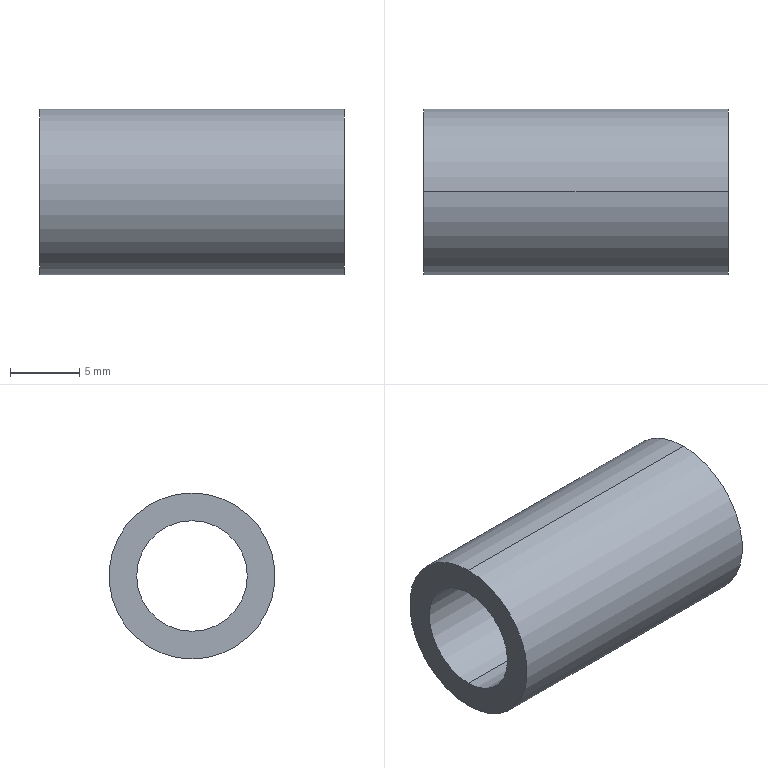Part | SolidWorks | features Revolution 1 | 1 solid | 6 faces | box 22 x 12 x 12 mm | volume 1382 mm3 | cylinder 4 | plane 2 | commonest cylinder face diameters 8 x2 12 x2
STEP:
#1=CARTESIAN_POINT('',(22.,0.,6.));
#2=VERTEX_POINT('',#1);
#3=CARTESIAN_POINT('',(22.,0.,-6.));
#4=VERTEX_POINT('',#3);
#5=CARTESIAN_POINT('',(22.,0.,0.));
#6=DIRECTION('',(-1.,0.,0.));
#7=DIRECTION('',(0.,0.,1.));
#8=AXIS2_PLACEMENT_3D('',#5,#6,#7);
#9=CIRCLE('',#8,6.);
#10=EDGE_CURVE('',#2,#4,#9,.T.);
#11=ORIENTED_EDGE('',*,*,#10,.T.);
#12=CARTESIAN_POINT('',(0.,0.,-6.));
#13=VERTEX_POINT('',#12);
#14=CARTESIAN_POINT('',(-539.036,0.,-6.));
#15=DIRECTION('',(-1.,0.,0.));
#16=VECTOR('',#15,1000.);
#17=LINE('',#14,#16);
#18=EDGE_CURVE('',#4,#13,#17,.T.);
#19=ORIENTED_EDGE('',*,*,#18,.T.);
#20=CARTESIAN_POINT('',(0.,0.,6.));
#21=VERTEX_POINT('',#20);
#22=CARTESIAN_POINT('',(0.,0.,0.));
#23=DIRECTION('',(-1.,0.,0.));
#24=DIRECTION('',(0.,0.,1.));
#25=AXIS2_PLACEMENT_3D('',#22,#23,#24);
#26=CIRCLE('',#25,6.);
#27=EDGE_CURVE('',#21,#13,#26,.T.);
#28=ORIENTED_EDGE('',*,*,#27,.F.);
#29=CARTESIAN_POINT('',(-539.036,0.,6.));
#30=DIRECTION('',(-1.,0.,0.));
#31=VECTOR('',#30,1000.);
#32=LINE('',#29,#31);
#33=EDGE_CURVE('',#2,#21,#32,.T.);
#34=ORIENTED_EDGE('',*,*,#33,.F.);
#35=EDGE_LOOP('',(#11,#19,#28,#34));
#36=FACE_OUTER_BOUND('',#35,.T.);
#37=CARTESIAN_POINT('',(-539.036,0.,0.));
#38=DIRECTION('',(-1.,0.,0.));
#39=DIRECTION('',(0.,0.,1.));
#40=AXIS2_PLACEMENT_3D('',#37,#38,#39);
#41=CYLINDRICAL_SURFACE('',#40,6.);
#42=ADVANCED_FACE('',(#36),#41,.T.);
#43=CARTESIAN_POINT('',(22.,0.,-4.));
#44=VERTEX_POINT('',#43);
#45=CARTESIAN_POINT('',(22.,0.,4.));
#46=VERTEX_POINT('',#45);
#47=CARTESIAN_POINT('',(22.,0.,0.));
#48=DIRECTION('',(-1.,0.,0.));
#49=DIRECTION('',(0.,0.,1.));
#50=AXIS2_PLACEMENT_3D('',#47,#48,#49);
#51=CIRCLE('',#50,4.);
#52=EDGE_CURVE('',#44,#46,#51,.T.);
#53=ORIENTED_EDGE('',*,*,#52,.F.);
#54=CARTESIAN_POINT('',(0.,0.,-4.));
#55=VERTEX_POINT('',#54);
#56=CARTESIAN_POINT('',(-539.036,0.,-4.));
#57=DIRECTION('',(-1.,0.,0.));
#58=VECTOR('',#57,1000.);
#59=LINE('',#56,#58);
#60=EDGE_CURVE('',#44,#55,#59,.T.);
#61=ORIENTED_EDGE('',*,*,#60,.T.);
#62=CARTESIAN_POINT('',(0.,0.,4.));
#63=VERTEX_POINT('',#62);
#64=CARTESIAN_POINT('',(0.,0.,0.));
#65=DIRECTION('',(-1.,0.,0.));
#66=DIRECTION('',(0.,0.,1.));
#67=AXIS2_PLACEMENT_3D('',#64,#65,#66);
#68=CIRCLE('',#67,4.);
#69=EDGE_CURVE('',#55,#63,#68,.T.);
#70=ORIENTED_EDGE('',*,*,#69,.T.);
#71=CARTESIAN_POINT('',(-539.036,0.,4.));
#72=DIRECTION('',(-1.,0.,0.));
#73=VECTOR('',#72,1000.);
#74=LINE('',#71,#73);
#75=EDGE_CURVE('',#46,#63,#74,.T.);
#76=ORIENTED_EDGE('',*,*,#75,.F.);
#77=EDGE_LOOP('',(#53,#61,#70,#76));
#78=FACE_OUTER_BOUND('',#77,.T.);
#79=CARTESIAN_POINT('',(-539.036,0.,0.));
#80=DIRECTION('',(-1.,0.,0.));
#81=DIRECTION('',(0.,0.,1.));
#82=AXIS2_PLACEMENT_3D('',#79,#80,#81);
#83=CYLINDRICAL_SURFACE('',#82,4.);
#84=ADVANCED_FACE('',(#78),#83,.F.);
#85=ORIENTED_EDGE('',*,*,#60,.F.);
#86=CARTESIAN_POINT('',(22.,0.,0.));
#87=DIRECTION('',(-1.,0.,0.));
#88=DIRECTION('',(0.,0.,1.));
#89=AXIS2_PLACEMENT_3D('',#86,#87,#88);
#90=CIRCLE('',#89,4.);
#91=EDGE_CURVE('',#46,#44,#90,.T.);
#92=ORIENTED_EDGE('',*,*,#91,.F.);
#93=ORIENTED_EDGE('',*,*,#75,.T.);
#94=CARTESIAN_POINT('',(0.,0.,0.));
#95=DIRECTION('',(-1.,0.,0.));
#96=DIRECTION('',(0.,0.,1.));
#97=AXIS2_PLACEMENT_3D('',#94,#95,#96);
#98=CIRCLE('',#97,4.);
#99=EDGE_CURVE('',#63,#55,#98,.T.);
#100=ORIENTED_EDGE('',*,*,#99,.T.);
#101=EDGE_LOOP('',(#85,#92,#93,#100));
#102=FACE_OUTER_BOUND('',#101,.T.);
#103=CARTESIAN_POINT('',(-539.036,0.,0.));
#104=DIRECTION('',(-1.,0.,0.));
#105=DIRECTION('',(0.,0.,1.));
#106=AXIS2_PLACEMENT_3D('',#103,#104,#105);
#107=CYLINDRICAL_SURFACE('',#106,4.);
#108=ADVANCED_FACE('',(#102),#107,.F.);
#109=ORIENTED_EDGE('',*,*,#99,.F.);
#110=ORIENTED_EDGE('',*,*,#69,.F.);
#111=EDGE_LOOP('',(#109,#110));
#112=FACE_BOUND('',#111,.T.);
#113=ORIENTED_EDGE('',*,*,#27,.T.);
#114=CARTESIAN_POINT('',(0.,0.,0.));
#115=DIRECTION('',(-1.,0.,0.));
#116=DIRECTION('',(0.,0.,1.));
#117=AXIS2_PLACEMENT_3D('',#114,#115,#116);
#118=CIRCLE('',#117,6.);
#119=EDGE_CURVE('',#13,#21,#118,.T.);
#120=ORIENTED_EDGE('',*,*,#119,.T.);
#121=EDGE_LOOP('',(#113,#120));
#122=FACE_OUTER_BOUND('',#121,.T.);
#123=CARTESIAN_POINT('',(0.,4.,0.));
#124=DIRECTION('',(1.,0.,0.));
#125=DIRECTION('',(0.,0.,-1.));
#126=AXIS2_PLACEMENT_3D('',#123,#124,#125);
#127=PLANE('',#126);
#128=ADVANCED_FACE('',(#112,#122),#127,.F.);
#129=ORIENTED_EDGE('',*,*,#18,.F.);
#130=CARTESIAN_POINT('',(22.,0.,0.));
#131=DIRECTION('',(-1.,0.,0.));
#132=DIRECTION('',(0.,0.,1.));
#133=AXIS2_PLACEMENT_3D('',#130,#131,#132);
#134=CIRCLE('',#133,6.);
#135=EDGE_CURVE('',#4,#2,#134,.T.);
#136=ORIENTED_EDGE('',*,*,#135,.T.);
#137=ORIENTED_EDGE('',*,*,#33,.T.);
#138=ORIENTED_EDGE('',*,*,#119,.F.);
#139=EDGE_LOOP('',(#129,#136,#137,#138));
#140=FACE_OUTER_BOUND('',#139,.T.);
#141=CARTESIAN_POINT('',(-539.036,0.,0.));
#142=DIRECTION('',(-1.,0.,0.));
#143=DIRECTION('',(0.,0.,1.));
#144=AXIS2_PLACEMENT_3D('',#141,#142,#143);
#145=CYLINDRICAL_SURFACE('',#144,6.);
#146=ADVANCED_FACE('',(#140),#145,.T.);
#147=ORIENTED_EDGE('',*,*,#10,.F.);
#148=ORIENTED_EDGE('',*,*,#135,.F.);
#149=EDGE_LOOP('',(#147,#148));
#150=FACE_OUTER_BOUND('',#149,.T.);
#151=ORIENTED_EDGE('',*,*,#91,.T.);
#152=ORIENTED_EDGE('',*,*,#52,.T.);
#153=EDGE_LOOP('',(#151,#152));
#154=FACE_BOUND('',#153,.T.);
#155=CARTESIAN_POINT('',(22.,6.,0.));
#156=DIRECTION('',(-1.,0.,0.));
#157=DIRECTION('',(0.,0.,1.));
#158=AXIS2_PLACEMENT_3D('',#155,#156,#157);
#159=PLANE('',#158);
#160=ADVANCED_FACE('',(#150,#154),#159,.F.);
#161=CLOSED_SHELL('',(#42,#84,#108,#128,#146,#160));
#162=MANIFOLD_SOLID_BREP('',#161);
#163=CARTESIAN_POINT('',(0.,0.,0.));
#164=DIRECTION('',(0.,0.,1.));
#165=DIRECTION('',(1.,0.,0.));
#166=AXIS2_PLACEMENT_3D('',#163,#164,#165);
#167=(LENGTH_UNIT()NAMED_UNIT(*)SI_UNIT(.MILLI.,.METRE.));
#168=UNCERTAINTY_MEASURE_WITH_UNIT(LENGTH_MEASURE(0.00001),#167,'','');
#169=(NAMED_UNIT(*)PLANE_ANGLE_UNIT()SI_UNIT($,.RADIAN.));
#170=(NAMED_UNIT(*)SI_UNIT($,.STERADIAN.)SOLID_ANGLE_UNIT());
#171=(GEOMETRIC_REPRESENTATION_CONTEXT(3)GLOBAL_UNCERTAINTY_ASSIGNED_CONTEXT((#168))GLOBAL_UNIT_ASSIGNED_CONTEXT((#167,#169,#170))REPRESENTATION_CONTEXT('',''));
#172=ADVANCED_BREP_SHAPE_REPRESENTATION('',(#162,#166),#171);